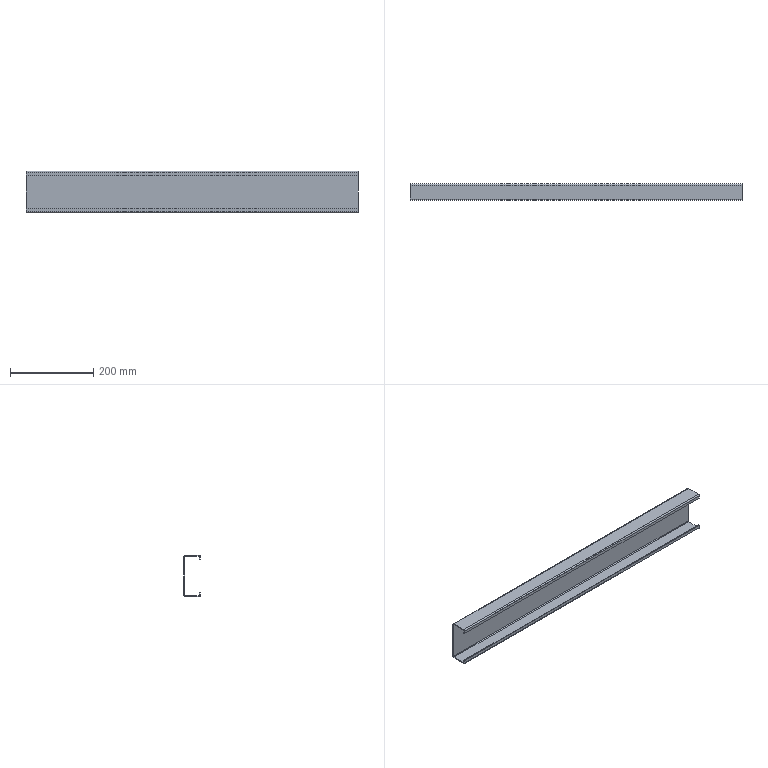Part | SolidWorks | features EdgeFlange 2, FlatPattern 1, SMBaseFlange 1, SheetMetal 1 | 1 solid | 38 faces | box 800 x 40 x 100 mm | volume 300333 mm3 | plane 30 | cylinder 8 | commonest cylinder face diameters 2 x2 4 x2 6 x2 8 x2
STEP:
#1=CARTESIAN_POINT('',(-674.379,-37.,-2.));
#2=VERTEX_POINT('',#1);
#3=CARTESIAN_POINT('',(-674.379,-4.,-2.));
#4=VERTEX_POINT('',#3);
#5=CARTESIAN_POINT('',(-674.379,0.,-2.));
#6=DIRECTION('',(0.,1.,0.));
#7=VECTOR('',#6,1000.);
#8=LINE('',#5,#7);
#9=EDGE_CURVE('',#2,#4,#8,.T.);
#10=ORIENTED_EDGE('',*,*,#9,.F.);
#11=CARTESIAN_POINT('',(-674.379,-37.,0.));
#12=VERTEX_POINT('',#11);
#13=CARTESIAN_POINT('',(-674.379,-37.,-2.));
#14=DIRECTION('',(0.,0.,1.));
#15=VECTOR('',#14,1000.);
#16=LINE('',#13,#15);
#17=EDGE_CURVE('',#2,#12,#16,.T.);
#18=ORIENTED_EDGE('',*,*,#17,.T.);
#19=CARTESIAN_POINT('',(-674.379,-4.,0.));
#20=VERTEX_POINT('',#19);
#21=CARTESIAN_POINT('',(-674.379,-2.,0.));
#22=DIRECTION('',(0.,1.,0.));
#23=VECTOR('',#22,1000.);
#24=LINE('',#21,#23);
#25=EDGE_CURVE('',#12,#20,#24,.T.);
#26=ORIENTED_EDGE('',*,*,#25,.T.);
#27=CARTESIAN_POINT('',(-674.379,-4.,-2.));
#28=DIRECTION('',(0.,0.,1.));
#29=VECTOR('',#28,1000.);
#30=LINE('',#27,#29);
#31=EDGE_CURVE('',#4,#20,#30,.T.);
#32=ORIENTED_EDGE('',*,*,#31,.F.);
#33=EDGE_LOOP('',(#10,#18,#26,#32));
#34=FACE_OUTER_BOUND('',#33,.T.);
#35=CARTESIAN_POINT('',(-674.379,-2.,0.));
#36=DIRECTION('',(-1.,0.,0.));
#37=DIRECTION('',(0.,0.,1.));
#38=AXIS2_PLACEMENT_3D('',#35,#36,#37);
#39=PLANE('',#38);
#40=ADVANCED_FACE('',(#34),#39,.T.);
#41=ORIENTED_EDGE('',*,*,#25,.F.);
#42=CARTESIAN_POINT('',(125.621,-37.,0.));
#43=VERTEX_POINT('',#42);
#44=CARTESIAN_POINT('',(-674.379,-37.,0.));
#45=DIRECTION('',(1.,0.,0.));
#46=VECTOR('',#45,1000.);
#47=LINE('',#44,#46);
#48=EDGE_CURVE('',#12,#43,#47,.T.);
#49=ORIENTED_EDGE('',*,*,#48,.T.);
#50=CARTESIAN_POINT('',(125.621,-4.,0.));
#51=VERTEX_POINT('',#50);
#52=CARTESIAN_POINT('',(125.621,-40.,0.));
#53=DIRECTION('',(0.,-1.,0.));
#54=VECTOR('',#53,1000.);
#55=LINE('',#52,#54);
#56=EDGE_CURVE('',#51,#43,#55,.T.);
#57=ORIENTED_EDGE('',*,*,#56,.F.);
#58=CARTESIAN_POINT('',(0.,-4.,0.));
#59=DIRECTION('',(-1.,0.,0.));
#60=VECTOR('',#59,1000.);
#61=LINE('',#58,#60);
#62=EDGE_CURVE('',#51,#20,#61,.T.);
#63=ORIENTED_EDGE('',*,*,#62,.T.);
#64=EDGE_LOOP('',(#41,#49,#57,#63));
#65=FACE_OUTER_BOUND('',#64,.T.);
#66=CARTESIAN_POINT('',(0.,0.,0.));
#67=DIRECTION('',(0.,0.,1.));
#68=DIRECTION('',(0.,-1.,0.));
#69=AXIS2_PLACEMENT_3D('',#66,#67,#68);
#70=PLANE('',#69);
#71=ADVANCED_FACE('',(#65),#70,.T.);
#72=CARTESIAN_POINT('',(125.621,-37.,-2.));
#73=VERTEX_POINT('',#72);
#74=CARTESIAN_POINT('',(-674.379,-37.,-2.));
#75=DIRECTION('',(1.,0.,0.));
#76=VECTOR('',#75,1000.);
#77=LINE('',#74,#76);
#78=EDGE_CURVE('',#2,#73,#77,.T.);
#79=ORIENTED_EDGE('',*,*,#78,.F.);
#80=ORIENTED_EDGE('',*,*,#9,.T.);
#81=CARTESIAN_POINT('',(125.621,-4.,-2.));
#82=VERTEX_POINT('',#81);
#83=CARTESIAN_POINT('',(125.621,-4.,-2.));
#84=DIRECTION('',(-1.,0.,0.));
#85=VECTOR('',#84,1000.);
#86=LINE('',#83,#85);
#87=EDGE_CURVE('',#82,#4,#86,.T.);
#88=ORIENTED_EDGE('',*,*,#87,.F.);
#89=CARTESIAN_POINT('',(125.621,0.,-2.));
#90=DIRECTION('',(0.,-1.,0.));
#91=VECTOR('',#90,1000.);
#92=LINE('',#89,#91);
#93=EDGE_CURVE('',#82,#73,#92,.T.);
#94=ORIENTED_EDGE('',*,*,#93,.T.);
#95=EDGE_LOOP('',(#79,#80,#88,#94));
#96=FACE_OUTER_BOUND('',#95,.T.);
#97=CARTESIAN_POINT('',(0.,0.,-2.));
#98=DIRECTION('',(0.,0.,1.));
#99=DIRECTION('',(0.,-1.,0.));
#100=AXIS2_PLACEMENT_3D('',#97,#98,#99);
#101=PLANE('',#100);
#102=ADVANCED_FACE('',(#96),#101,.F.);
#103=CARTESIAN_POINT('',(125.621,-37.,-98.));
#104=VERTEX_POINT('',#103);
#105=CARTESIAN_POINT('',(125.621,-4.,-98.));
#106=VERTEX_POINT('',#105);
#107=CARTESIAN_POINT('',(125.621,0.,-98.));
#108=DIRECTION('',(0.,1.,0.));
#109=VECTOR('',#108,1000.);
#110=LINE('',#107,#109);
#111=EDGE_CURVE('',#104,#106,#110,.T.);
#112=ORIENTED_EDGE('',*,*,#111,.F.);
#113=CARTESIAN_POINT('',(125.621,-37.,-100.));
#114=VERTEX_POINT('',#113);
#115=CARTESIAN_POINT('',(125.621,-37.,-98.));
#116=DIRECTION('',(0.,0.,-1.));
#117=VECTOR('',#116,1000.);
#118=LINE('',#115,#117);
#119=EDGE_CURVE('',#104,#114,#118,.T.);
#120=ORIENTED_EDGE('',*,*,#119,.T.);
#121=CARTESIAN_POINT('',(125.621,-4.,-100.));
#122=VERTEX_POINT('',#121);
#123=CARTESIAN_POINT('',(125.621,-2.,-100.));
#124=DIRECTION('',(0.,1.,0.));
#125=VECTOR('',#124,1000.);
#126=LINE('',#123,#125);
#127=EDGE_CURVE('',#114,#122,#126,.T.);
#128=ORIENTED_EDGE('',*,*,#127,.T.);
#129=CARTESIAN_POINT('',(125.621,-4.,-98.));
#130=DIRECTION('',(0.,0.,-1.));
#131=VECTOR('',#130,1000.);
#132=LINE('',#129,#131);
#133=EDGE_CURVE('',#106,#122,#132,.T.);
#134=ORIENTED_EDGE('',*,*,#133,.F.);
#135=EDGE_LOOP('',(#112,#120,#128,#134));
#136=FACE_OUTER_BOUND('',#135,.T.);
#137=CARTESIAN_POINT('',(125.621,-2.,-100.));
#138=DIRECTION('',(1.,0.,0.));
#139=DIRECTION('',(0.,0.,-1.));
#140=AXIS2_PLACEMENT_3D('',#137,#138,#139);
#141=PLANE('',#140);
#142=ADVANCED_FACE('',(#136),#141,.T.);
#143=ORIENTED_EDGE('',*,*,#127,.F.);
#144=CARTESIAN_POINT('',(-674.379,-37.,-100.));
#145=VERTEX_POINT('',#144);
#146=CARTESIAN_POINT('',(125.621,-37.,-100.));
#147=DIRECTION('',(-1.,0.,0.));
#148=VECTOR('',#147,1000.);
#149=LINE('',#146,#148);
#150=EDGE_CURVE('',#114,#145,#149,.T.);
#151=ORIENTED_EDGE('',*,*,#150,.T.);
#152=CARTESIAN_POINT('',(-674.379,-4.,-100.));
#153=VERTEX_POINT('',#152);
#154=CARTESIAN_POINT('',(-674.379,-40.,-100.));
#155=DIRECTION('',(0.,-1.,0.));
#156=VECTOR('',#155,1000.);
#157=LINE('',#154,#156);
#158=EDGE_CURVE('',#153,#145,#157,.T.);
#159=ORIENTED_EDGE('',*,*,#158,.F.);
#160=CARTESIAN_POINT('',(0.,-4.,-100.));
#161=DIRECTION('',(1.,0.,0.));
#162=VECTOR('',#161,1000.);
#163=LINE('',#160,#162);
#164=EDGE_CURVE('',#153,#122,#163,.T.);
#165=ORIENTED_EDGE('',*,*,#164,.T.);
#166=EDGE_LOOP('',(#143,#151,#159,#165));
#167=FACE_OUTER_BOUND('',#166,.T.);
#168=CARTESIAN_POINT('',(0.,0.,-100.));
#169=DIRECTION('',(0.,0.,-1.));
#170=DIRECTION('',(0.,1.,0.));
#171=AXIS2_PLACEMENT_3D('',#168,#169,#170);
#172=PLANE('',#171);
#173=ADVANCED_FACE('',(#167),#172,.T.);
#174=CARTESIAN_POINT('',(-674.379,-37.,-98.));
#175=VERTEX_POINT('',#174);
#176=CARTESIAN_POINT('',(125.621,-37.,-98.));
#177=DIRECTION('',(-1.,0.,0.));
#178=VECTOR('',#177,1000.);
#179=LINE('',#176,#178);
#180=EDGE_CURVE('',#104,#175,#179,.T.);
#181=ORIENTED_EDGE('',*,*,#180,.F.);
#182=ORIENTED_EDGE('',*,*,#111,.T.);
#183=CARTESIAN_POINT('',(-674.379,-4.,-98.));
#184=VERTEX_POINT('',#183);
#185=CARTESIAN_POINT('',(-674.379,-4.,-98.));
#186=DIRECTION('',(1.,0.,0.));
#187=VECTOR('',#186,1000.);
#188=LINE('',#185,#187);
#189=EDGE_CURVE('',#184,#106,#188,.T.);
#190=ORIENTED_EDGE('',*,*,#189,.F.);
#191=CARTESIAN_POINT('',(-674.379,0.,-98.));
#192=DIRECTION('',(0.,-1.,0.));
#193=VECTOR('',#192,1000.);
#194=LINE('',#191,#193);
#195=EDGE_CURVE('',#184,#175,#194,.T.);
#196=ORIENTED_EDGE('',*,*,#195,.T.);
#197=EDGE_LOOP('',(#181,#182,#190,#196));
#198=FACE_OUTER_BOUND('',#197,.T.);
#199=CARTESIAN_POINT('',(0.,0.,-98.));
#200=DIRECTION('',(0.,0.,-1.));
#201=DIRECTION('',(0.,1.,0.));
#202=AXIS2_PLACEMENT_3D('',#199,#200,#201);
#203=PLANE('',#202);
#204=ADVANCED_FACE('',(#198),#203,.F.);
#205=CARTESIAN_POINT('',(125.621,-2.,-96.));
#206=VERTEX_POINT('',#205);
#207=CARTESIAN_POINT('',(-674.379,-2.,-96.));
#208=VERTEX_POINT('',#207);
#209=CARTESIAN_POINT('',(125.621,-2.,-96.));
#210=DIRECTION('',(-1.,0.,0.));
#211=VECTOR('',#210,1000.);
#212=LINE('',#209,#211);
#213=EDGE_CURVE('',#206,#208,#212,.T.);
#214=ORIENTED_EDGE('',*,*,#213,.F.);
#215=CARTESIAN_POINT('',(125.621,-2.,-4.));
#216=VERTEX_POINT('',#215);
#217=CARTESIAN_POINT('',(125.621,-2.,-100.));
#218=DIRECTION('',(0.,0.,-1.));
#219=VECTOR('',#218,1000.);
#220=LINE('',#217,#219);
#221=EDGE_CURVE('',#216,#206,#220,.T.);
#222=ORIENTED_EDGE('',*,*,#221,.F.);
#223=CARTESIAN_POINT('',(-674.379,-2.,-4.));
#224=VERTEX_POINT('',#223);
#225=CARTESIAN_POINT('',(-674.379,-2.,-4.));
#226=DIRECTION('',(1.,0.,0.));
#227=VECTOR('',#226,1000.);
#228=LINE('',#225,#227);
#229=EDGE_CURVE('',#224,#216,#228,.T.);
#230=ORIENTED_EDGE('',*,*,#229,.F.);
#231=CARTESIAN_POINT('',(-674.379,-2.,-100.));
#232=DIRECTION('',(0.,0.,1.));
#233=VECTOR('',#232,1000.);
#234=LINE('',#231,#233);
#235=EDGE_CURVE('',#208,#224,#234,.T.);
#236=ORIENTED_EDGE('',*,*,#235,.F.);
#237=EDGE_LOOP('',(#214,#222,#230,#236));
#238=FACE_OUTER_BOUND('',#237,.T.);
#239=CARTESIAN_POINT('',(0.,-2.,0.));
#240=DIRECTION('',(0.,1.,0.));
#241=DIRECTION('',(0.,0.,1.));
#242=AXIS2_PLACEMENT_3D('',#239,#240,#241);
#243=PLANE('',#242);
#244=ADVANCED_FACE('',(#238),#243,.F.);
#245=CARTESIAN_POINT('',(125.621,0.,-4.));
#246=VERTEX_POINT('',#245);
#247=CARTESIAN_POINT('',(125.621,0.,-96.));
#248=VERTEX_POINT('',#247);
#249=CARTESIAN_POINT('',(125.621,0.,-100.));
#250=DIRECTION('',(0.,0.,-1.));
#251=VECTOR('',#250,1000.);
#252=LINE('',#249,#251);
#253=EDGE_CURVE('',#246,#248,#252,.T.);
#254=ORIENTED_EDGE('',*,*,#253,.T.);
#255=CARTESIAN_POINT('',(-674.379,0.,-96.));
#256=VERTEX_POINT('',#255);
#257=CARTESIAN_POINT('',(125.621,0.,-96.));
#258=DIRECTION('',(-1.,0.,0.));
#259=VECTOR('',#258,1000.);
#260=LINE('',#257,#259);
#261=EDGE_CURVE('',#248,#256,#260,.T.);
#262=ORIENTED_EDGE('',*,*,#261,.T.);
#263=CARTESIAN_POINT('',(-674.379,0.,-4.));
#264=VERTEX_POINT('',#263);
#265=CARTESIAN_POINT('',(-674.379,0.,-100.));
#266=DIRECTION('',(0.,0.,1.));
#267=VECTOR('',#266,1000.);
#268=LINE('',#265,#267);
#269=EDGE_CURVE('',#256,#264,#268,.T.);
#270=ORIENTED_EDGE('',*,*,#269,.T.);
#271=CARTESIAN_POINT('',(-674.379,0.,-4.));
#272=DIRECTION('',(1.,0.,0.));
#273=VECTOR('',#272,1000.);
#274=LINE('',#271,#273);
#275=EDGE_CURVE('',#264,#246,#274,.T.);
#276=ORIENTED_EDGE('',*,*,#275,.T.);
#277=EDGE_LOOP('',(#254,#262,#270,#276));
#278=FACE_OUTER_BOUND('',#277,.T.);
#279=CARTESIAN_POINT('',(0.,0.,0.));
#280=DIRECTION('',(0.,1.,0.));
#281=DIRECTION('',(0.,0.,1.));
#282=AXIS2_PLACEMENT_3D('',#279,#280,#281);
#283=PLANE('',#282);
#284=ADVANCED_FACE('',(#278),#283,.T.);
#285=ORIENTED_EDGE('',*,*,#221,.T.);
#286=CARTESIAN_POINT('',(125.621,-2.,-96.));
#287=DIRECTION('',(0.,1.,0.));
#288=VECTOR('',#287,1000.);
#289=LINE('',#286,#288);
#290=EDGE_CURVE('',#206,#248,#289,.T.);
#291=ORIENTED_EDGE('',*,*,#290,.T.);
#292=ORIENTED_EDGE('',*,*,#253,.F.);
#293=CARTESIAN_POINT('',(125.621,-2.,-4.));
#294=DIRECTION('',(0.,1.,0.));
#295=VECTOR('',#294,1000.);
#296=LINE('',#293,#295);
#297=EDGE_CURVE('',#216,#246,#296,.T.);
#298=ORIENTED_EDGE('',*,*,#297,.F.);
#299=EDGE_LOOP('',(#285,#291,#292,#298));
#300=FACE_OUTER_BOUND('',#299,.T.);
#301=CARTESIAN_POINT('',(125.621,-2.,-100.));
#302=DIRECTION('',(1.,0.,0.));
#303=DIRECTION('',(0.,0.,-1.));
#304=AXIS2_PLACEMENT_3D('',#301,#302,#303);
#305=PLANE('',#304);
#306=ADVANCED_FACE('',(#300),#305,.T.);
#307=CARTESIAN_POINT('',(-674.379,-2.,-96.));
#308=DIRECTION('',(0.,1.,0.));
#309=VECTOR('',#308,1000.);
#310=LINE('',#307,#309);
#311=EDGE_CURVE('',#208,#256,#310,.T.);
#312=ORIENTED_EDGE('',*,*,#311,.F.);
#313=ORIENTED_EDGE('',*,*,#235,.T.);
#314=CARTESIAN_POINT('',(-674.379,-2.,-4.));
#315=DIRECTION('',(0.,1.,0.));
#316=VECTOR('',#315,1000.);
#317=LINE('',#314,#316);
#318=EDGE_CURVE('',#224,#264,#317,.T.);
#319=ORIENTED_EDGE('',*,*,#318,.T.);
#320=ORIENTED_EDGE('',*,*,#269,.F.);
#321=EDGE_LOOP('',(#312,#313,#319,#320));
#322=FACE_OUTER_BOUND('',#321,.T.);
#323=CARTESIAN_POINT('',(-674.379,-2.,-100.));
#324=DIRECTION('',(-1.,0.,0.));
#325=DIRECTION('',(0.,0.,1.));
#326=AXIS2_PLACEMENT_3D('',#323,#324,#325);
#327=PLANE('',#326);
#328=ADVANCED_FACE('',(#322),#327,.T.);
#329=CARTESIAN_POINT('',(125.621,-4.,0.));
#330=DIRECTION('',(0.,0.,1.));
#331=VECTOR('',#330,1000.);
#332=LINE('',#329,#331);
#333=EDGE_CURVE('',#82,#51,#332,.T.);
#334=ORIENTED_EDGE('',*,*,#333,.F.);
#335=CARTESIAN_POINT('',(125.621,-4.,-4.));
#336=DIRECTION('',(1.,0.,0.));
#337=DIRECTION('',(0.,0.,1.));
#338=AXIS2_PLACEMENT_3D('',#335,#336,#337);
#339=CIRCLE('',#338,2.);
#340=EDGE_CURVE('',#216,#82,#339,.T.);
#341=ORIENTED_EDGE('',*,*,#340,.F.);
#342=ORIENTED_EDGE('',*,*,#297,.T.);
#343=CARTESIAN_POINT('',(125.621,-4.,-4.));
#344=DIRECTION('',(1.,0.,0.));
#345=DIRECTION('',(0.,0.,1.));
#346=AXIS2_PLACEMENT_3D('',#343,#344,#345);
#347=CIRCLE('',#346,4.);
#348=EDGE_CURVE('',#246,#51,#347,.T.);
#349=ORIENTED_EDGE('',*,*,#348,.T.);
#350=EDGE_LOOP('',(#334,#341,#342,#349));
#351=FACE_OUTER_BOUND('',#350,.T.);
#352=CARTESIAN_POINT('',(125.621,-4.,-4.));
#353=DIRECTION('',(1.,0.,0.));
#354=DIRECTION('',(0.,0.,-1.));
#355=AXIS2_PLACEMENT_3D('',#352,#353,#354);
#356=PLANE('',#355);
#357=ADVANCED_FACE('',(#351),#356,.T.);
#358=CARTESIAN_POINT('',(-674.379,-4.,-4.));
#359=DIRECTION('',(-1.,0.,0.));
#360=DIRECTION('',(0.,0.,1.));
#361=AXIS2_PLACEMENT_3D('',#358,#359,#360);
#362=CIRCLE('',#361,2.);
#363=EDGE_CURVE('',#4,#224,#362,.T.);
#364=ORIENTED_EDGE('',*,*,#363,.F.);
#365=ORIENTED_EDGE('',*,*,#31,.T.);
#366=CARTESIAN_POINT('',(-674.379,-4.,-4.));
#367=DIRECTION('',(-1.,0.,0.));
#368=DIRECTION('',(0.,0.,1.));
#369=AXIS2_PLACEMENT_3D('',#366,#367,#368);
#370=CIRCLE('',#369,4.);
#371=EDGE_CURVE('',#20,#264,#370,.T.);
#372=ORIENTED_EDGE('',*,*,#371,.T.);
#373=ORIENTED_EDGE('',*,*,#318,.F.);
#374=EDGE_LOOP('',(#364,#365,#372,#373));
#375=FACE_OUTER_BOUND('',#374,.T.);
#376=CARTESIAN_POINT('',(-674.379,-4.,-4.));
#377=DIRECTION('',(1.,0.,0.));
#378=DIRECTION('',(0.,0.,-1.));
#379=AXIS2_PLACEMENT_3D('',#376,#377,#378);
#380=PLANE('',#379);
#381=ADVANCED_FACE('',(#375),#380,.F.);
#382=ORIENTED_EDGE('',*,*,#275,.F.);
#383=ORIENTED_EDGE('',*,*,#371,.F.);
#384=ORIENTED_EDGE('',*,*,#62,.F.);
#385=ORIENTED_EDGE('',*,*,#348,.F.);
#386=EDGE_LOOP('',(#382,#383,#384,#385));
#387=FACE_OUTER_BOUND('',#386,.T.);
#388=CARTESIAN_POINT('',(-674.379,-4.,-4.));
#389=DIRECTION('',(-1.,0.,0.));
#390=DIRECTION('',(0.,0.,1.));
#391=AXIS2_PLACEMENT_3D('',#388,#389,#390);
#392=CYLINDRICAL_SURFACE('',#391,4.);
#393=ADVANCED_FACE('',(#387),#392,.T.);
#394=ORIENTED_EDGE('',*,*,#229,.T.);
#395=ORIENTED_EDGE('',*,*,#340,.T.);
#396=ORIENTED_EDGE('',*,*,#87,.T.);
#397=ORIENTED_EDGE('',*,*,#363,.T.);
#398=EDGE_LOOP('',(#394,#395,#396,#397));
#399=FACE_OUTER_BOUND('',#398,.T.);
#400=CARTESIAN_POINT('',(-674.379,-4.,-4.));
#401=DIRECTION('',(-1.,0.,0.));
#402=DIRECTION('',(0.,0.,1.));
#403=AXIS2_PLACEMENT_3D('',#400,#401,#402);
#404=CYLINDRICAL_SURFACE('',#403,2.);
#405=ADVANCED_FACE('',(#399),#404,.F.);
#406=CARTESIAN_POINT('',(125.621,-37.,-2.));
#407=DIRECTION('',(0.,0.,1.));
#408=VECTOR('',#407,1000.);
#409=LINE('',#406,#408);
#410=EDGE_CURVE('',#73,#43,#409,.T.);
#411=ORIENTED_EDGE('',*,*,#410,.F.);
#412=ORIENTED_EDGE('',*,*,#93,.F.);
#413=ORIENTED_EDGE('',*,*,#333,.T.);
#414=ORIENTED_EDGE('',*,*,#56,.T.);
#415=EDGE_LOOP('',(#411,#412,#413,#414));
#416=FACE_OUTER_BOUND('',#415,.T.);
#417=CARTESIAN_POINT('',(125.621,-40.,0.));
#418=DIRECTION('',(1.,0.,0.));
#419=DIRECTION('',(0.,0.,-1.));
#420=AXIS2_PLACEMENT_3D('',#417,#418,#419);
#421=PLANE('',#420);
#422=ADVANCED_FACE('',(#416),#421,.T.);
#423=CARTESIAN_POINT('',(-674.379,-4.,-100.));
#424=DIRECTION('',(0.,0.,-1.));
#425=VECTOR('',#424,1000.);
#426=LINE('',#423,#425);
#427=EDGE_CURVE('',#184,#153,#426,.T.);
#428=ORIENTED_EDGE('',*,*,#427,.F.);
#429=CARTESIAN_POINT('',(-674.379,-4.,-96.));
#430=DIRECTION('',(-1.,0.,0.));
#431=DIRECTION('',(0.,0.,-1.));
#432=AXIS2_PLACEMENT_3D('',#429,#430,#431);
#433=CIRCLE('',#432,2.);
#434=EDGE_CURVE('',#208,#184,#433,.T.);
#435=ORIENTED_EDGE('',*,*,#434,.F.);
#436=ORIENTED_EDGE('',*,*,#311,.T.);
#437=CARTESIAN_POINT('',(-674.379,-4.,-96.));
#438=DIRECTION('',(-1.,0.,0.));
#439=DIRECTION('',(0.,0.,-1.));
#440=AXIS2_PLACEMENT_3D('',#437,#438,#439);
#441=CIRCLE('',#440,4.);
#442=EDGE_CURVE('',#256,#153,#441,.T.);
#443=ORIENTED_EDGE('',*,*,#442,.T.);
#444=EDGE_LOOP('',(#428,#435,#436,#443));
#445=FACE_OUTER_BOUND('',#444,.T.);
#446=CARTESIAN_POINT('',(-674.379,-4.,-96.));
#447=DIRECTION('',(-1.,0.,0.));
#448=DIRECTION('',(0.,0.,1.));
#449=AXIS2_PLACEMENT_3D('',#446,#447,#448);
#450=PLANE('',#449);
#451=ADVANCED_FACE('',(#445),#450,.T.);
#452=CARTESIAN_POINT('',(125.621,-4.,-96.));
#453=DIRECTION('',(1.,0.,0.));
#454=DIRECTION('',(0.,0.,-1.));
#455=AXIS2_PLACEMENT_3D('',#452,#453,#454);
#456=CIRCLE('',#455,2.);
#457=EDGE_CURVE('',#106,#206,#456,.T.);
#458=ORIENTED_EDGE('',*,*,#457,.F.);
#459=ORIENTED_EDGE('',*,*,#133,.T.);
#460=CARTESIAN_POINT('',(125.621,-4.,-96.));
#461=DIRECTION('',(1.,0.,0.));
#462=DIRECTION('',(0.,0.,-1.));
#463=AXIS2_PLACEMENT_3D('',#460,#461,#462);
#464=CIRCLE('',#463,4.);
#465=EDGE_CURVE('',#122,#248,#464,.T.);
#466=ORIENTED_EDGE('',*,*,#465,.T.);
#467=ORIENTED_EDGE('',*,*,#290,.F.);
#468=EDGE_LOOP('',(#458,#459,#466,#467));
#469=FACE_OUTER_BOUND('',#468,.T.);
#470=CARTESIAN_POINT('',(125.621,-4.,-96.));
#471=DIRECTION('',(-1.,0.,0.));
#472=DIRECTION('',(0.,0.,1.));
#473=AXIS2_PLACEMENT_3D('',#470,#471,#472);
#474=PLANE('',#473);
#475=ADVANCED_FACE('',(#469),#474,.F.);
#476=ORIENTED_EDGE('',*,*,#261,.F.);
#477=ORIENTED_EDGE('',*,*,#465,.F.);
#478=ORIENTED_EDGE('',*,*,#164,.F.);
#479=ORIENTED_EDGE('',*,*,#442,.F.);
#480=EDGE_LOOP('',(#476,#477,#478,#479));
#481=FACE_OUTER_BOUND('',#480,.T.);
#482=CARTESIAN_POINT('',(125.621,-4.,-96.));
#483=DIRECTION('',(1.,0.,0.));
#484=DIRECTION('',(0.,0.,-1.));
#485=AXIS2_PLACEMENT_3D('',#482,#483,#484);
#486=CYLINDRICAL_SURFACE('',#485,4.);
#487=ADVANCED_FACE('',(#481),#486,.T.);
#488=ORIENTED_EDGE('',*,*,#213,.T.);
#489=ORIENTED_EDGE('',*,*,#434,.T.);
#490=ORIENTED_EDGE('',*,*,#189,.T.);
#491=ORIENTED_EDGE('',*,*,#457,.T.);
#492=EDGE_LOOP('',(#488,#489,#490,#491));
#493=FACE_OUTER_BOUND('',#492,.T.);
#494=CARTESIAN_POINT('',(125.621,-4.,-96.));
#495=DIRECTION('',(1.,0.,0.));
#496=DIRECTION('',(0.,0.,-1.));
#497=AXIS2_PLACEMENT_3D('',#494,#495,#496);
#498=CYLINDRICAL_SURFACE('',#497,2.);
#499=ADVANCED_FACE('',(#493),#498,.F.);
#500=CARTESIAN_POINT('',(-674.379,-37.,-98.));
#501=DIRECTION('',(0.,0.,-1.));
#502=VECTOR('',#501,1000.);
#503=LINE('',#500,#502);
#504=EDGE_CURVE('',#175,#145,#503,.T.);
#505=ORIENTED_EDGE('',*,*,#504,.F.);
#506=ORIENTED_EDGE('',*,*,#195,.F.);
#507=ORIENTED_EDGE('',*,*,#427,.T.);
#508=ORIENTED_EDGE('',*,*,#158,.T.);
#509=EDGE_LOOP('',(#505,#506,#507,#508));
#510=FACE_OUTER_BOUND('',#509,.T.);
#511=CARTESIAN_POINT('',(-674.379,-40.,-100.));
#512=DIRECTION('',(-1.,0.,0.));
#513=DIRECTION('',(0.,0.,1.));
#514=AXIS2_PLACEMENT_3D('',#511,#512,#513);
#515=PLANE('',#514);
#516=ADVANCED_FACE('',(#510),#515,.T.);
#517=CARTESIAN_POINT('',(-674.379,-38.,-97.));
#518=VERTEX_POINT('',#517);
#519=CARTESIAN_POINT('',(-674.379,-40.,-97.));
#520=VERTEX_POINT('',#519);
#521=CARTESIAN_POINT('',(-674.379,-40.,-97.));
#522=DIRECTION('',(0.,-1.,0.));
#523=VECTOR('',#522,1000.);
#524=LINE('',#521,#523);
#525=EDGE_CURVE('',#518,#520,#524,.T.);
#526=ORIENTED_EDGE('',*,*,#525,.F.);
#527=CARTESIAN_POINT('',(-674.379,-37.,-97.));
#528=DIRECTION('',(-1.,0.,0.));
#529=DIRECTION('',(0.,0.,-1.));
#530=AXIS2_PLACEMENT_3D('',#527,#528,#529);
#531=CIRCLE('',#530,1.);
#532=EDGE_CURVE('',#175,#518,#531,.T.);
#533=ORIENTED_EDGE('',*,*,#532,.F.);
#534=ORIENTED_EDGE('',*,*,#504,.T.);
#535=CARTESIAN_POINT('',(-674.379,-37.,-97.));
#536=DIRECTION('',(-1.,0.,0.));
#537=DIRECTION('',(0.,0.,-1.));
#538=AXIS2_PLACEMENT_3D('',#535,#536,#537);
#539=CIRCLE('',#538,3.);
#540=EDGE_CURVE('',#145,#520,#539,.T.);
#541=ORIENTED_EDGE('',*,*,#540,.T.);
#542=EDGE_LOOP('',(#526,#533,#534,#541));
#543=FACE_OUTER_BOUND('',#542,.T.);
#544=CARTESIAN_POINT('',(-674.379,-37.,-97.));
#545=DIRECTION('',(-1.,0.,0.));
#546=DIRECTION('',(0.,0.,1.));
#547=AXIS2_PLACEMENT_3D('',#544,#545,#546);
#548=PLANE('',#547);
#549=ADVANCED_FACE('',(#543),#548,.T.);
#550=CARTESIAN_POINT('',(125.621,-38.,-97.));
#551=VERTEX_POINT('',#550);
#552=CARTESIAN_POINT('',(125.621,-37.,-97.));
#553=DIRECTION('',(1.,0.,0.));
#554=DIRECTION('',(0.,0.,-1.));
#555=AXIS2_PLACEMENT_3D('',#552,#553,#554);
#556=CIRCLE('',#555,1.);
#557=EDGE_CURVE('',#551,#104,#556,.T.);
#558=ORIENTED_EDGE('',*,*,#557,.F.);
#559=CARTESIAN_POINT('',(125.621,-40.,-97.));
#560=VERTEX_POINT('',#559);
#561=CARTESIAN_POINT('',(125.621,-38.,-97.));
#562=DIRECTION('',(0.,-1.,0.));
#563=VECTOR('',#562,1000.);
#564=LINE('',#561,#563);
#565=EDGE_CURVE('',#551,#560,#564,.T.);
#566=ORIENTED_EDGE('',*,*,#565,.T.);
#567=CARTESIAN_POINT('',(125.621,-37.,-97.));
#568=DIRECTION('',(1.,0.,0.));
#569=DIRECTION('',(0.,0.,-1.));
#570=AXIS2_PLACEMENT_3D('',#567,#568,#569);
#571=CIRCLE('',#570,3.);
#572=EDGE_CURVE('',#560,#114,#571,.T.);
#573=ORIENTED_EDGE('',*,*,#572,.T.);
#574=ORIENTED_EDGE('',*,*,#119,.F.);
#575=EDGE_LOOP('',(#558,#566,#573,#574));
#576=FACE_OUTER_BOUND('',#575,.T.);
#577=CARTESIAN_POINT('',(125.621,-37.,-97.));
#578=DIRECTION('',(-1.,0.,0.));
#579=DIRECTION('',(0.,0.,1.));
#580=AXIS2_PLACEMENT_3D('',#577,#578,#579);
#581=PLANE('',#580);
#582=ADVANCED_FACE('',(#576),#581,.F.);
#583=ORIENTED_EDGE('',*,*,#150,.F.);
#584=ORIENTED_EDGE('',*,*,#572,.F.);
#585=CARTESIAN_POINT('',(-674.379,-40.,-97.));
#586=DIRECTION('',(-1.,0.,0.));
#587=VECTOR('',#586,1000.);
#588=LINE('',#585,#587);
#589=EDGE_CURVE('',#560,#520,#588,.T.);
#590=ORIENTED_EDGE('',*,*,#589,.T.);
#591=ORIENTED_EDGE('',*,*,#540,.F.);
#592=EDGE_LOOP('',(#583,#584,#590,#591));
#593=FACE_OUTER_BOUND('',#592,.T.);
#594=CARTESIAN_POINT('',(125.621,-37.,-97.));
#595=DIRECTION('',(1.,0.,0.));
#596=DIRECTION('',(0.,-1.,0.));
#597=AXIS2_PLACEMENT_3D('',#594,#595,#596);
#598=CYLINDRICAL_SURFACE('',#597,3.);
#599=ADVANCED_FACE('',(#593),#598,.T.);
#600=ORIENTED_EDGE('',*,*,#180,.T.);
#601=ORIENTED_EDGE('',*,*,#532,.T.);
#602=CARTESIAN_POINT('',(-674.379,-38.,-97.));
#603=DIRECTION('',(1.,0.,0.));
#604=VECTOR('',#603,1000.);
#605=LINE('',#602,#604);
#606=EDGE_CURVE('',#518,#551,#605,.T.);
#607=ORIENTED_EDGE('',*,*,#606,.T.);
#608=ORIENTED_EDGE('',*,*,#557,.T.);
#609=EDGE_LOOP('',(#600,#601,#607,#608));
#610=FACE_OUTER_BOUND('',#609,.T.);
#611=CARTESIAN_POINT('',(125.621,-37.,-97.));
#612=DIRECTION('',(1.,0.,0.));
#613=DIRECTION('',(0.,-1.,0.));
#614=AXIS2_PLACEMENT_3D('',#611,#612,#613);
#615=CYLINDRICAL_SURFACE('',#614,1.);
#616=ADVANCED_FACE('',(#610),#615,.F.);
#617=ORIENTED_EDGE('',*,*,#565,.F.);
#618=CARTESIAN_POINT('',(125.621,-38.,-90.));
#619=VERTEX_POINT('',#618);
#620=CARTESIAN_POINT('',(125.621,-38.,-90.));
#621=DIRECTION('',(0.,0.,1.));
#622=VECTOR('',#621,1000.);
#623=LINE('',#620,#622);
#624=EDGE_CURVE('',#551,#619,#623,.T.);
#625=ORIENTED_EDGE('',*,*,#624,.T.);
#626=CARTESIAN_POINT('',(125.621,-40.,-90.));
#627=VERTEX_POINT('',#626);
#628=CARTESIAN_POINT('',(125.621,-40.,-90.));
#629=DIRECTION('',(0.,1.,0.));
#630=VECTOR('',#629,1000.);
#631=LINE('',#628,#630);
#632=EDGE_CURVE('',#627,#619,#631,.T.);
#633=ORIENTED_EDGE('',*,*,#632,.F.);
#634=CARTESIAN_POINT('',(125.621,-40.,0.));
#635=DIRECTION('',(0.,0.,1.));
#636=VECTOR('',#635,1000.);
#637=LINE('',#634,#636);
#638=EDGE_CURVE('',#560,#627,#637,.T.);
#639=ORIENTED_EDGE('',*,*,#638,.F.);
#640=EDGE_LOOP('',(#617,#625,#633,#639));
#641=FACE_OUTER_BOUND('',#640,.T.);
#642=CARTESIAN_POINT('',(125.621,-40.,-90.));
#643=DIRECTION('',(-1.,0.,0.));
#644=DIRECTION('',(0.,0.,1.));
#645=AXIS2_PLACEMENT_3D('',#642,#643,#644);
#646=PLANE('',#645);
#647=ADVANCED_FACE('',(#641),#646,.F.);
#648=ORIENTED_EDGE('',*,*,#525,.T.);
#649=CARTESIAN_POINT('',(-674.379,-40.,-90.));
#650=VERTEX_POINT('',#649);
#651=CARTESIAN_POINT('',(-674.379,-40.,0.));
#652=DIRECTION('',(0.,0.,-1.));
#653=VECTOR('',#652,1000.);
#654=LINE('',#651,#653);
#655=EDGE_CURVE('',#650,#520,#654,.T.);
#656=ORIENTED_EDGE('',*,*,#655,.F.);
#657=CARTESIAN_POINT('',(-674.379,-38.,-90.));
#658=VERTEX_POINT('',#657);
#659=CARTESIAN_POINT('',(-674.379,-40.,-90.));
#660=DIRECTION('',(0.,1.,0.));
#661=VECTOR('',#660,1000.);
#662=LINE('',#659,#661);
#663=EDGE_CURVE('',#650,#658,#662,.T.);
#664=ORIENTED_EDGE('',*,*,#663,.T.);
#665=CARTESIAN_POINT('',(-674.379,-38.,-98.));
#666=DIRECTION('',(0.,0.,-1.));
#667=VECTOR('',#666,1000.);
#668=LINE('',#665,#667);
#669=EDGE_CURVE('',#658,#518,#668,.T.);
#670=ORIENTED_EDGE('',*,*,#669,.T.);
#671=EDGE_LOOP('',(#648,#656,#664,#670));
#672=FACE_OUTER_BOUND('',#671,.T.);
#673=CARTESIAN_POINT('',(-674.379,-40.,-98.));
#674=DIRECTION('',(1.,0.,0.));
#675=DIRECTION('',(0.,0.,-1.));
#676=AXIS2_PLACEMENT_3D('',#673,#674,#675);
#677=PLANE('',#676);
#678=ADVANCED_FACE('',(#672),#677,.F.);
#679=ORIENTED_EDGE('',*,*,#589,.F.);
#680=ORIENTED_EDGE('',*,*,#638,.T.);
#681=CARTESIAN_POINT('',(0.,-40.,-90.));
#682=DIRECTION('',(-1.,0.,0.));
#683=VECTOR('',#682,1000.);
#684=LINE('',#681,#683);
#685=EDGE_CURVE('',#627,#650,#684,.T.);
#686=ORIENTED_EDGE('',*,*,#685,.T.);
#687=ORIENTED_EDGE('',*,*,#655,.T.);
#688=EDGE_LOOP('',(#679,#680,#686,#687));
#689=FACE_OUTER_BOUND('',#688,.T.);
#690=CARTESIAN_POINT('',(0.,-40.,0.));
#691=DIRECTION('',(0.,1.,0.));
#692=DIRECTION('',(0.,0.,1.));
#693=AXIS2_PLACEMENT_3D('',#690,#691,#692);
#694=PLANE('',#693);
#695=ADVANCED_FACE('',(#689),#694,.F.);
#696=ORIENTED_EDGE('',*,*,#624,.F.);
#697=ORIENTED_EDGE('',*,*,#606,.F.);
#698=ORIENTED_EDGE('',*,*,#669,.F.);
#699=CARTESIAN_POINT('',(-674.379,-38.,-90.));
#700=DIRECTION('',(-1.,0.,0.));
#701=VECTOR('',#700,1000.);
#702=LINE('',#699,#701);
#703=EDGE_CURVE('',#619,#658,#702,.T.);
#704=ORIENTED_EDGE('',*,*,#703,.F.);
#705=EDGE_LOOP('',(#696,#697,#698,#704));
#706=FACE_OUTER_BOUND('',#705,.T.);
#707=CARTESIAN_POINT('',(0.,-38.,0.));
#708=DIRECTION('',(0.,1.,0.));
#709=DIRECTION('',(0.,0.,1.));
#710=AXIS2_PLACEMENT_3D('',#707,#708,#709);
#711=PLANE('',#710);
#712=ADVANCED_FACE('',(#706),#711,.T.);
#713=ORIENTED_EDGE('',*,*,#703,.T.);
#714=ORIENTED_EDGE('',*,*,#663,.F.);
#715=ORIENTED_EDGE('',*,*,#685,.F.);
#716=ORIENTED_EDGE('',*,*,#632,.T.);
#717=EDGE_LOOP('',(#713,#714,#715,#716));
#718=FACE_OUTER_BOUND('',#717,.T.);
#719=CARTESIAN_POINT('',(-674.379,-40.,-90.));
#720=DIRECTION('',(0.,0.,-1.));
#721=DIRECTION('',(0.,1.,0.));
#722=AXIS2_PLACEMENT_3D('',#719,#720,#721);
#723=PLANE('',#722);
#724=ADVANCED_FACE('',(#718),#723,.F.);
#725=CARTESIAN_POINT('',(125.621,-38.,-3.));
#726=VERTEX_POINT('',#725);
#727=CARTESIAN_POINT('',(125.621,-40.,-3.));
#728=VERTEX_POINT('',#727);
#729=CARTESIAN_POINT('',(125.621,-40.,-3.));
#730=DIRECTION('',(0.,-1.,0.));
#731=VECTOR('',#730,1000.);
#732=LINE('',#729,#731);
#733=EDGE_CURVE('',#726,#728,#732,.T.);
#734=ORIENTED_EDGE('',*,*,#733,.F.);
#735=CARTESIAN_POINT('',(125.621,-37.,-3.));
#736=DIRECTION('',(1.,0.,0.));
#737=DIRECTION('',(0.,0.,1.));
#738=AXIS2_PLACEMENT_3D('',#735,#736,#737);
#739=CIRCLE('',#738,1.);
#740=EDGE_CURVE('',#73,#726,#739,.T.);
#741=ORIENTED_EDGE('',*,*,#740,.F.);
#742=ORIENTED_EDGE('',*,*,#410,.T.);
#743=CARTESIAN_POINT('',(125.621,-37.,-3.));
#744=DIRECTION('',(1.,0.,0.));
#745=DIRECTION('',(0.,0.,1.));
#746=AXIS2_PLACEMENT_3D('',#743,#744,#745);
#747=CIRCLE('',#746,3.);
#748=EDGE_CURVE('',#43,#728,#747,.T.);
#749=ORIENTED_EDGE('',*,*,#748,.T.);
#750=EDGE_LOOP('',(#734,#741,#742,#749));
#751=FACE_OUTER_BOUND('',#750,.T.);
#752=CARTESIAN_POINT('',(125.621,-37.,-3.));
#753=DIRECTION('',(1.,0.,0.));
#754=DIRECTION('',(0.,0.,-1.));
#755=AXIS2_PLACEMENT_3D('',#752,#753,#754);
#756=PLANE('',#755);
#757=ADVANCED_FACE('',(#751),#756,.T.);
#758=CARTESIAN_POINT('',(-674.379,-38.,-3.));
#759=VERTEX_POINT('',#758);
#760=CARTESIAN_POINT('',(-674.379,-37.,-3.));
#761=DIRECTION('',(-1.,0.,0.));
#762=DIRECTION('',(0.,0.,1.));
#763=AXIS2_PLACEMENT_3D('',#760,#761,#762);
#764=CIRCLE('',#763,1.);
#765=EDGE_CURVE('',#759,#2,#764,.T.);
#766=ORIENTED_EDGE('',*,*,#765,.F.);
#767=CARTESIAN_POINT('',(-674.379,-40.,-3.));
#768=VERTEX_POINT('',#767);
#769=CARTESIAN_POINT('',(-674.379,-38.,-3.));
#770=DIRECTION('',(0.,-1.,0.));
#771=VECTOR('',#770,1000.);
#772=LINE('',#769,#771);
#773=EDGE_CURVE('',#759,#768,#772,.T.);
#774=ORIENTED_EDGE('',*,*,#773,.T.);
#775=CARTESIAN_POINT('',(-674.379,-37.,-3.));
#776=DIRECTION('',(-1.,0.,0.));
#777=DIRECTION('',(0.,0.,1.));
#778=AXIS2_PLACEMENT_3D('',#775,#776,#777);
#779=CIRCLE('',#778,3.);
#780=EDGE_CURVE('',#768,#12,#779,.T.);
#781=ORIENTED_EDGE('',*,*,#780,.T.);
#782=ORIENTED_EDGE('',*,*,#17,.F.);
#783=EDGE_LOOP('',(#766,#774,#781,#782));
#784=FACE_OUTER_BOUND('',#783,.T.);
#785=CARTESIAN_POINT('',(-674.379,-37.,-3.));
#786=DIRECTION('',(1.,0.,0.));
#787=DIRECTION('',(0.,0.,-1.));
#788=AXIS2_PLACEMENT_3D('',#785,#786,#787);
#789=PLANE('',#788);
#790=ADVANCED_FACE('',(#784),#789,.F.);
#791=ORIENTED_EDGE('',*,*,#48,.F.);
#792=ORIENTED_EDGE('',*,*,#780,.F.);
#793=CARTESIAN_POINT('',(125.621,-40.,-3.));
#794=DIRECTION('',(1.,0.,0.));
#795=VECTOR('',#794,1000.);
#796=LINE('',#793,#795);
#797=EDGE_CURVE('',#768,#728,#796,.T.);
#798=ORIENTED_EDGE('',*,*,#797,.T.);
#799=ORIENTED_EDGE('',*,*,#748,.F.);
#800=EDGE_LOOP('',(#791,#792,#798,#799));
#801=FACE_OUTER_BOUND('',#800,.T.);
#802=CARTESIAN_POINT('',(-674.379,-37.,-3.));
#803=DIRECTION('',(-1.,0.,0.));
#804=DIRECTION('',(0.,-1.,0.));
#805=AXIS2_PLACEMENT_3D('',#802,#803,#804);
#806=CYLINDRICAL_SURFACE('',#805,3.);
#807=ADVANCED_FACE('',(#801),#806,.T.);
#808=ORIENTED_EDGE('',*,*,#78,.T.);
#809=ORIENTED_EDGE('',*,*,#740,.T.);
#810=CARTESIAN_POINT('',(125.621,-38.,-3.));
#811=DIRECTION('',(-1.,0.,0.));
#812=VECTOR('',#811,1000.);
#813=LINE('',#810,#812);
#814=EDGE_CURVE('',#726,#759,#813,.T.);
#815=ORIENTED_EDGE('',*,*,#814,.T.);
#816=ORIENTED_EDGE('',*,*,#765,.T.);
#817=EDGE_LOOP('',(#808,#809,#815,#816));
#818=FACE_OUTER_BOUND('',#817,.T.);
#819=CARTESIAN_POINT('',(-674.379,-37.,-3.));
#820=DIRECTION('',(-1.,0.,0.));
#821=DIRECTION('',(0.,-1.,0.));
#822=AXIS2_PLACEMENT_3D('',#819,#820,#821);
#823=CYLINDRICAL_SURFACE('',#822,1.);
#824=ADVANCED_FACE('',(#818),#823,.F.);
#825=ORIENTED_EDGE('',*,*,#733,.T.);
#826=CARTESIAN_POINT('',(125.621,-40.,-10.));
#827=VERTEX_POINT('',#826);
#828=CARTESIAN_POINT('',(125.621,-40.,0.));
#829=DIRECTION('',(0.,0.,1.));
#830=VECTOR('',#829,1000.);
#831=LINE('',#828,#830);
#832=EDGE_CURVE('',#827,#728,#831,.T.);
#833=ORIENTED_EDGE('',*,*,#832,.F.);
#834=CARTESIAN_POINT('',(125.621,-38.,-10.));
#835=VERTEX_POINT('',#834);
#836=CARTESIAN_POINT('',(125.621,-40.,-10.));
#837=DIRECTION('',(0.,1.,0.));
#838=VECTOR('',#837,1000.);
#839=LINE('',#836,#838);
#840=EDGE_CURVE('',#827,#835,#839,.T.);
#841=ORIENTED_EDGE('',*,*,#840,.T.);
#842=CARTESIAN_POINT('',(125.621,-38.,-2.));
#843=DIRECTION('',(0.,0.,1.));
#844=VECTOR('',#843,1000.);
#845=LINE('',#842,#844);
#846=EDGE_CURVE('',#835,#726,#845,.T.);
#847=ORIENTED_EDGE('',*,*,#846,.T.);
#848=EDGE_LOOP('',(#825,#833,#841,#847));
#849=FACE_OUTER_BOUND('',#848,.T.);
#850=CARTESIAN_POINT('',(125.621,-40.,-2.));
#851=DIRECTION('',(-1.,0.,0.));
#852=DIRECTION('',(0.,0.,1.));
#853=AXIS2_PLACEMENT_3D('',#850,#851,#852);
#854=PLANE('',#853);
#855=ADVANCED_FACE('',(#849),#854,.F.);
#856=ORIENTED_EDGE('',*,*,#773,.F.);
#857=CARTESIAN_POINT('',(-674.379,-38.,-10.));
#858=VERTEX_POINT('',#857);
#859=CARTESIAN_POINT('',(-674.379,-38.,-10.));
#860=DIRECTION('',(0.,0.,-1.));
#861=VECTOR('',#860,1000.);
#862=LINE('',#859,#861);
#863=EDGE_CURVE('',#759,#858,#862,.T.);
#864=ORIENTED_EDGE('',*,*,#863,.T.);
#865=CARTESIAN_POINT('',(-674.379,-40.,-10.));
#866=VERTEX_POINT('',#865);
#867=CARTESIAN_POINT('',(-674.379,-40.,-10.));
#868=DIRECTION('',(0.,1.,0.));
#869=VECTOR('',#868,1000.);
#870=LINE('',#867,#869);
#871=EDGE_CURVE('',#866,#858,#870,.T.);
#872=ORIENTED_EDGE('',*,*,#871,.F.);
#873=CARTESIAN_POINT('',(-674.379,-40.,0.));
#874=DIRECTION('',(0.,0.,-1.));
#875=VECTOR('',#874,1000.);
#876=LINE('',#873,#875);
#877=EDGE_CURVE('',#768,#866,#876,.T.);
#878=ORIENTED_EDGE('',*,*,#877,.F.);
#879=EDGE_LOOP('',(#856,#864,#872,#878));
#880=FACE_OUTER_BOUND('',#879,.T.);
#881=CARTESIAN_POINT('',(-674.379,-40.,-10.));
#882=DIRECTION('',(1.,0.,0.));
#883=DIRECTION('',(0.,0.,-1.));
#884=AXIS2_PLACEMENT_3D('',#881,#882,#883);
#885=PLANE('',#884);
#886=ADVANCED_FACE('',(#880),#885,.F.);
#887=ORIENTED_EDGE('',*,*,#797,.F.);
#888=ORIENTED_EDGE('',*,*,#877,.T.);
#889=CARTESIAN_POINT('',(0.,-40.,-10.));
#890=DIRECTION('',(1.,0.,0.));
#891=VECTOR('',#890,1000.);
#892=LINE('',#889,#891);
#893=EDGE_CURVE('',#866,#827,#892,.T.);
#894=ORIENTED_EDGE('',*,*,#893,.T.);
#895=ORIENTED_EDGE('',*,*,#832,.T.);
#896=EDGE_LOOP('',(#887,#888,#894,#895));
#897=FACE_OUTER_BOUND('',#896,.T.);
#898=CARTESIAN_POINT('',(0.,-40.,0.));
#899=DIRECTION('',(0.,1.,0.));
#900=DIRECTION('',(0.,0.,1.));
#901=AXIS2_PLACEMENT_3D('',#898,#899,#900);
#902=PLANE('',#901);
#903=ADVANCED_FACE('',(#897),#902,.F.);
#904=ORIENTED_EDGE('',*,*,#863,.F.);
#905=ORIENTED_EDGE('',*,*,#814,.F.);
#906=ORIENTED_EDGE('',*,*,#846,.F.);
#907=CARTESIAN_POINT('',(125.621,-38.,-10.));
#908=DIRECTION('',(1.,0.,0.));
#909=VECTOR('',#908,1000.);
#910=LINE('',#907,#909);
#911=EDGE_CURVE('',#858,#835,#910,.T.);
#912=ORIENTED_EDGE('',*,*,#911,.F.);
#913=EDGE_LOOP('',(#904,#905,#906,#912));
#914=FACE_OUTER_BOUND('',#913,.T.);
#915=CARTESIAN_POINT('',(0.,-38.,0.));
#916=DIRECTION('',(0.,1.,0.));
#917=DIRECTION('',(0.,0.,1.));
#918=AXIS2_PLACEMENT_3D('',#915,#916,#917);
#919=PLANE('',#918);
#920=ADVANCED_FACE('',(#914),#919,.T.);
#921=ORIENTED_EDGE('',*,*,#911,.T.);
#922=ORIENTED_EDGE('',*,*,#840,.F.);
#923=ORIENTED_EDGE('',*,*,#893,.F.);
#924=ORIENTED_EDGE('',*,*,#871,.T.);
#925=EDGE_LOOP('',(#921,#922,#923,#924));
#926=FACE_OUTER_BOUND('',#925,.T.);
#927=CARTESIAN_POINT('',(125.621,-40.,-10.));
#928=DIRECTION('',(0.,0.,1.));
#929=DIRECTION('',(0.,-1.,0.));
#930=AXIS2_PLACEMENT_3D('',#927,#928,#929);
#931=PLANE('',#930);
#932=ADVANCED_FACE('',(#926),#931,.F.);
#933=CLOSED_SHELL('',(#40,#71,#102,#142,#173,#204,#244,#284,#306,#328,#357,#381,#393,#405,#422,#451,#475,#487,#499,#516,#549,#582,#599,#616,#647,#678,#695,#712,#724,#757,#790,#807,#824,#855,#886,#903,#920,#932));
#934=MANIFOLD_SOLID_BREP('',#933);
#935=CARTESIAN_POINT('',(0.,0.,0.));
#936=DIRECTION('',(0.,0.,1.));
#937=DIRECTION('',(1.,0.,0.));
#938=AXIS2_PLACEMENT_3D('',#935,#936,#937);
#939=(LENGTH_UNIT()NAMED_UNIT(*)SI_UNIT(.MILLI.,.METRE.));
#940=UNCERTAINTY_MEASURE_WITH_UNIT(LENGTH_MEASURE(0.00001),#939,'','');
#941=(NAMED_UNIT(*)PLANE_ANGLE_UNIT()SI_UNIT($,.RADIAN.));
#942=(NAMED_UNIT(*)SI_UNIT($,.STERADIAN.)SOLID_ANGLE_UNIT());
#943=(GEOMETRIC_REPRESENTATION_CONTEXT(3)GLOBAL_UNCERTAINTY_ASSIGNED_CONTEXT((#940))GLOBAL_UNIT_ASSIGNED_CONTEXT((#939,#941,#942))REPRESENTATION_CONTEXT('',''));
#944=ADVANCED_BREP_SHAPE_REPRESENTATION('',(#934,#938),#943);